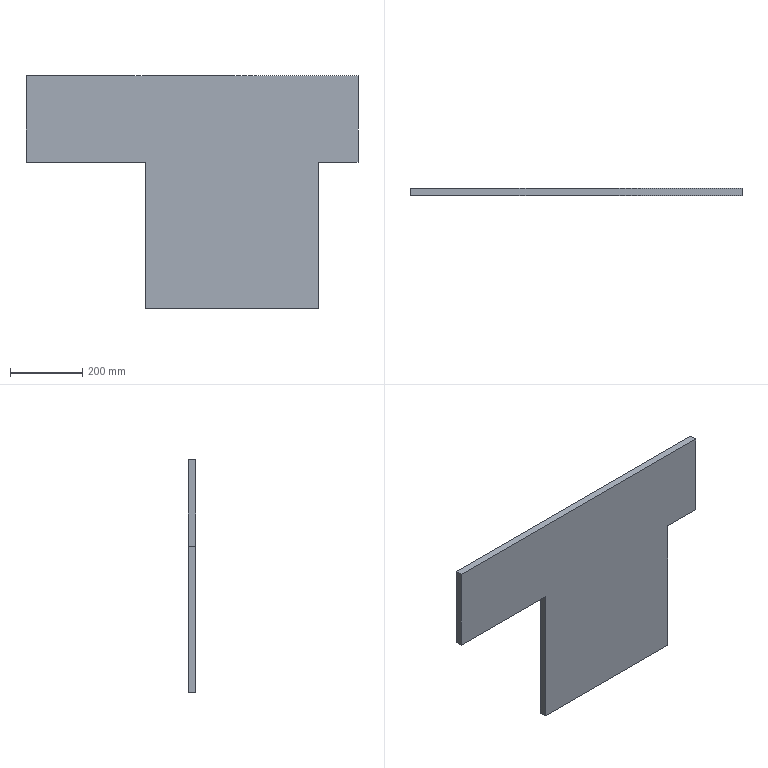Part | SolidWorks | features Extrusion 1 | 1 solid | 10 faces | box 920 x 20 x 645 mm | volume 8304000 mm3 | plane 10
STEP:
#1=CARTESIAN_POINT('',(590.,0.,655.));
#2=VERTEX_POINT('',#1);
#3=CARTESIAN_POINT('',(590.,0.,415.));
#4=VERTEX_POINT('',#3);
#5=CARTESIAN_POINT('',(590.,0.,655.));
#6=DIRECTION('',(0.,0.,-1.));
#7=VECTOR('',#6,1000.);
#8=LINE('',#5,#7);
#9=EDGE_CURVE('',#2,#4,#8,.T.);
#10=ORIENTED_EDGE('',*,*,#9,.T.);
#11=CARTESIAN_POINT('',(590.,20.,415.));
#12=VERTEX_POINT('',#11);
#13=CARTESIAN_POINT('',(590.,20.,415.));
#14=DIRECTION('',(0.,-1.,0.));
#15=VECTOR('',#14,1000.);
#16=LINE('',#13,#15);
#17=EDGE_CURVE('',#12,#4,#16,.T.);
#18=ORIENTED_EDGE('',*,*,#17,.F.);
#19=CARTESIAN_POINT('',(590.,20.,655.));
#20=VERTEX_POINT('',#19);
#21=CARTESIAN_POINT('',(590.,20.,655.));
#22=DIRECTION('',(0.,0.,-1.));
#23=VECTOR('',#22,1000.);
#24=LINE('',#21,#23);
#25=EDGE_CURVE('',#20,#12,#24,.T.);
#26=ORIENTED_EDGE('',*,*,#25,.F.);
#27=CARTESIAN_POINT('',(590.,20.,655.));
#28=DIRECTION('',(0.,-1.,0.));
#29=VECTOR('',#28,1000.);
#30=LINE('',#27,#29);
#31=EDGE_CURVE('',#20,#2,#30,.T.);
#32=ORIENTED_EDGE('',*,*,#31,.T.);
#33=EDGE_LOOP('',(#10,#18,#26,#32));
#34=FACE_OUTER_BOUND('',#33,.T.);
#35=CARTESIAN_POINT('',(590.,20.,655.));
#36=DIRECTION('',(-1.,0.,0.));
#37=DIRECTION('',(0.,0.,1.));
#38=AXIS2_PLACEMENT_3D('',#35,#36,#37);
#39=PLANE('',#38);
#40=ADVANCED_FACE('',(#34),#39,.F.);
#41=CARTESIAN_POINT('',(480.,0.,415.));
#42=VERTEX_POINT('',#41);
#43=CARTESIAN_POINT('',(590.,0.,415.));
#44=DIRECTION('',(-1.,0.,0.));
#45=VECTOR('',#44,1000.);
#46=LINE('',#43,#45);
#47=EDGE_CURVE('',#4,#42,#46,.T.);
#48=ORIENTED_EDGE('',*,*,#47,.T.);
#49=CARTESIAN_POINT('',(480.,20.,415.));
#50=VERTEX_POINT('',#49);
#51=CARTESIAN_POINT('',(480.,20.,415.));
#52=DIRECTION('',(0.,-1.,0.));
#53=VECTOR('',#52,1000.);
#54=LINE('',#51,#53);
#55=EDGE_CURVE('',#50,#42,#54,.T.);
#56=ORIENTED_EDGE('',*,*,#55,.F.);
#57=CARTESIAN_POINT('',(590.,20.,415.));
#58=DIRECTION('',(-1.,0.,0.));
#59=VECTOR('',#58,1000.);
#60=LINE('',#57,#59);
#61=EDGE_CURVE('',#12,#50,#60,.T.);
#62=ORIENTED_EDGE('',*,*,#61,.F.);
#63=ORIENTED_EDGE('',*,*,#17,.T.);
#64=EDGE_LOOP('',(#48,#56,#62,#63));
#65=FACE_OUTER_BOUND('',#64,.T.);
#66=CARTESIAN_POINT('',(590.,20.,415.));
#67=DIRECTION('',(0.,0.,1.));
#68=DIRECTION('',(1.,0.,0.));
#69=AXIS2_PLACEMENT_3D('',#66,#67,#68);
#70=PLANE('',#69);
#71=ADVANCED_FACE('',(#65),#70,.F.);
#72=CARTESIAN_POINT('',(480.,0.,10.));
#73=VERTEX_POINT('',#72);
#74=CARTESIAN_POINT('',(480.,0.,10.));
#75=DIRECTION('',(0.,0.,-1.));
#76=VECTOR('',#75,1000.);
#77=LINE('',#74,#76);
#78=EDGE_CURVE('',#42,#73,#77,.T.);
#79=ORIENTED_EDGE('',*,*,#78,.T.);
#80=CARTESIAN_POINT('',(480.,20.,10.));
#81=VERTEX_POINT('',#80);
#82=CARTESIAN_POINT('',(480.,20.,10.));
#83=DIRECTION('',(0.,-1.,0.));
#84=VECTOR('',#83,1000.);
#85=LINE('',#82,#84);
#86=EDGE_CURVE('',#81,#73,#85,.T.);
#87=ORIENTED_EDGE('',*,*,#86,.F.);
#88=CARTESIAN_POINT('',(480.,20.,10.));
#89=DIRECTION('',(0.,0.,-1.));
#90=VECTOR('',#89,1000.);
#91=LINE('',#88,#90);
#92=EDGE_CURVE('',#50,#81,#91,.T.);
#93=ORIENTED_EDGE('',*,*,#92,.F.);
#94=ORIENTED_EDGE('',*,*,#55,.T.);
#95=EDGE_LOOP('',(#79,#87,#93,#94));
#96=FACE_OUTER_BOUND('',#95,.T.);
#97=CARTESIAN_POINT('',(480.,20.,10.));
#98=DIRECTION('',(-1.,0.,0.));
#99=DIRECTION('',(0.,0.,1.));
#100=AXIS2_PLACEMENT_3D('',#97,#98,#99);
#101=PLANE('',#100);
#102=ADVANCED_FACE('',(#96),#101,.F.);
#103=CARTESIAN_POINT('',(0.,0.,10.));
#104=VERTEX_POINT('',#103);
#105=CARTESIAN_POINT('',(480.,0.,10.));
#106=DIRECTION('',(-1.,0.,0.));
#107=VECTOR('',#106,1000.);
#108=LINE('',#105,#107);
#109=EDGE_CURVE('',#73,#104,#108,.T.);
#110=ORIENTED_EDGE('',*,*,#109,.T.);
#111=CARTESIAN_POINT('',(0.,20.,10.));
#112=VERTEX_POINT('',#111);
#113=CARTESIAN_POINT('',(0.,20.,10.));
#114=DIRECTION('',(0.,-1.,0.));
#115=VECTOR('',#114,1000.);
#116=LINE('',#113,#115);
#117=EDGE_CURVE('',#112,#104,#116,.T.);
#118=ORIENTED_EDGE('',*,*,#117,.F.);
#119=CARTESIAN_POINT('',(480.,20.,10.));
#120=DIRECTION('',(-1.,0.,0.));
#121=VECTOR('',#120,1000.);
#122=LINE('',#119,#121);
#123=EDGE_CURVE('',#81,#112,#122,.T.);
#124=ORIENTED_EDGE('',*,*,#123,.F.);
#125=ORIENTED_EDGE('',*,*,#86,.T.);
#126=EDGE_LOOP('',(#110,#118,#124,#125));
#127=FACE_OUTER_BOUND('',#126,.T.);
#128=CARTESIAN_POINT('',(480.,20.,10.));
#129=DIRECTION('',(0.,0.,1.));
#130=DIRECTION('',(1.,0.,0.));
#131=AXIS2_PLACEMENT_3D('',#128,#129,#130);
#132=PLANE('',#131);
#133=ADVANCED_FACE('',(#127),#132,.F.);
#134=CARTESIAN_POINT('',(0.,0.,415.));
#135=VERTEX_POINT('',#134);
#136=CARTESIAN_POINT('',(0.,0.,415.));
#137=DIRECTION('',(0.,0.,1.));
#138=VECTOR('',#137,1000.);
#139=LINE('',#136,#138);
#140=EDGE_CURVE('',#104,#135,#139,.T.);
#141=ORIENTED_EDGE('',*,*,#140,.T.);
#142=CARTESIAN_POINT('',(0.,20.,415.));
#143=VERTEX_POINT('',#142);
#144=CARTESIAN_POINT('',(0.,20.,415.));
#145=DIRECTION('',(0.,-1.,0.));
#146=VECTOR('',#145,1000.);
#147=LINE('',#144,#146);
#148=EDGE_CURVE('',#143,#135,#147,.T.);
#149=ORIENTED_EDGE('',*,*,#148,.F.);
#150=CARTESIAN_POINT('',(0.,20.,415.));
#151=DIRECTION('',(0.,0.,1.));
#152=VECTOR('',#151,1000.);
#153=LINE('',#150,#152);
#154=EDGE_CURVE('',#112,#143,#153,.T.);
#155=ORIENTED_EDGE('',*,*,#154,.F.);
#156=ORIENTED_EDGE('',*,*,#117,.T.);
#157=EDGE_LOOP('',(#141,#149,#155,#156));
#158=FACE_OUTER_BOUND('',#157,.T.);
#159=CARTESIAN_POINT('',(0.,20.,415.));
#160=DIRECTION('',(1.,0.,0.));
#161=DIRECTION('',(0.,0.,-1.));
#162=AXIS2_PLACEMENT_3D('',#159,#160,#161);
#163=PLANE('',#162);
#164=ADVANCED_FACE('',(#158),#163,.F.);
#165=CARTESIAN_POINT('',(-330.,0.,415.));
#166=VERTEX_POINT('',#165);
#167=CARTESIAN_POINT('',(0.,0.,415.));
#168=DIRECTION('',(-1.,0.,0.));
#169=VECTOR('',#168,1000.);
#170=LINE('',#167,#169);
#171=EDGE_CURVE('',#135,#166,#170,.T.);
#172=ORIENTED_EDGE('',*,*,#171,.T.);
#173=CARTESIAN_POINT('',(-330.,20.,415.));
#174=VERTEX_POINT('',#173);
#175=CARTESIAN_POINT('',(-330.,20.,415.));
#176=DIRECTION('',(0.,-1.,0.));
#177=VECTOR('',#176,1000.);
#178=LINE('',#175,#177);
#179=EDGE_CURVE('',#174,#166,#178,.T.);
#180=ORIENTED_EDGE('',*,*,#179,.F.);
#181=CARTESIAN_POINT('',(0.,20.,415.));
#182=DIRECTION('',(-1.,0.,0.));
#183=VECTOR('',#182,1000.);
#184=LINE('',#181,#183);
#185=EDGE_CURVE('',#143,#174,#184,.T.);
#186=ORIENTED_EDGE('',*,*,#185,.F.);
#187=ORIENTED_EDGE('',*,*,#148,.T.);
#188=EDGE_LOOP('',(#172,#180,#186,#187));
#189=FACE_OUTER_BOUND('',#188,.T.);
#190=CARTESIAN_POINT('',(0.,20.,415.));
#191=DIRECTION('',(0.,0.,1.));
#192=DIRECTION('',(1.,0.,0.));
#193=AXIS2_PLACEMENT_3D('',#190,#191,#192);
#194=PLANE('',#193);
#195=ADVANCED_FACE('',(#189),#194,.F.);
#196=CARTESIAN_POINT('',(-330.,0.,655.));
#197=VERTEX_POINT('',#196);
#198=CARTESIAN_POINT('',(-330.,0.,415.));
#199=DIRECTION('',(0.,0.,1.));
#200=VECTOR('',#199,1000.);
#201=LINE('',#198,#200);
#202=EDGE_CURVE('',#166,#197,#201,.T.);
#203=ORIENTED_EDGE('',*,*,#202,.T.);
#204=CARTESIAN_POINT('',(-330.,20.,655.));
#205=VERTEX_POINT('',#204);
#206=CARTESIAN_POINT('',(-330.,20.,655.));
#207=DIRECTION('',(0.,-1.,0.));
#208=VECTOR('',#207,1000.);
#209=LINE('',#206,#208);
#210=EDGE_CURVE('',#205,#197,#209,.T.);
#211=ORIENTED_EDGE('',*,*,#210,.F.);
#212=CARTESIAN_POINT('',(-330.,20.,415.));
#213=DIRECTION('',(0.,0.,1.));
#214=VECTOR('',#213,1000.);
#215=LINE('',#212,#214);
#216=EDGE_CURVE('',#174,#205,#215,.T.);
#217=ORIENTED_EDGE('',*,*,#216,.F.);
#218=ORIENTED_EDGE('',*,*,#179,.T.);
#219=EDGE_LOOP('',(#203,#211,#217,#218));
#220=FACE_OUTER_BOUND('',#219,.T.);
#221=CARTESIAN_POINT('',(-330.,20.,415.));
#222=DIRECTION('',(1.,0.,0.));
#223=DIRECTION('',(0.,0.,-1.));
#224=AXIS2_PLACEMENT_3D('',#221,#222,#223);
#225=PLANE('',#224);
#226=ADVANCED_FACE('',(#220),#225,.F.);
#227=CARTESIAN_POINT('',(-330.,0.,655.));
#228=DIRECTION('',(1.,0.,0.));
#229=VECTOR('',#228,1000.);
#230=LINE('',#227,#229);
#231=EDGE_CURVE('',#197,#2,#230,.T.);
#232=ORIENTED_EDGE('',*,*,#231,.T.);
#233=ORIENTED_EDGE('',*,*,#31,.F.);
#234=CARTESIAN_POINT('',(-330.,20.,655.));
#235=DIRECTION('',(1.,0.,0.));
#236=VECTOR('',#235,1000.);
#237=LINE('',#234,#236);
#238=EDGE_CURVE('',#205,#20,#237,.T.);
#239=ORIENTED_EDGE('',*,*,#238,.F.);
#240=ORIENTED_EDGE('',*,*,#210,.T.);
#241=EDGE_LOOP('',(#232,#233,#239,#240));
#242=FACE_OUTER_BOUND('',#241,.T.);
#243=CARTESIAN_POINT('',(-330.,20.,655.));
#244=DIRECTION('',(0.,0.,-1.));
#245=DIRECTION('',(-1.,0.,0.));
#246=AXIS2_PLACEMENT_3D('',#243,#244,#245);
#247=PLANE('',#246);
#248=ADVANCED_FACE('',(#242),#247,.F.);
#249=ORIENTED_EDGE('',*,*,#25,.T.);
#250=ORIENTED_EDGE('',*,*,#61,.T.);
#251=ORIENTED_EDGE('',*,*,#92,.T.);
#252=ORIENTED_EDGE('',*,*,#123,.T.);
#253=ORIENTED_EDGE('',*,*,#154,.T.);
#254=ORIENTED_EDGE('',*,*,#185,.T.);
#255=ORIENTED_EDGE('',*,*,#216,.T.);
#256=ORIENTED_EDGE('',*,*,#238,.T.);
#257=EDGE_LOOP('',(#249,#250,#251,#252,#253,#254,#255,#256));
#258=FACE_OUTER_BOUND('',#257,.T.);
#259=CARTESIAN_POINT('',(0.,20.,0.));
#260=DIRECTION('',(0.,1.,0.));
#261=DIRECTION('',(0.,0.,1.));
#262=AXIS2_PLACEMENT_3D('',#259,#260,#261);
#263=PLANE('',#262);
#264=ADVANCED_FACE('',(#258),#263,.T.);
#265=ORIENTED_EDGE('',*,*,#9,.F.);
#266=ORIENTED_EDGE('',*,*,#231,.F.);
#267=ORIENTED_EDGE('',*,*,#202,.F.);
#268=ORIENTED_EDGE('',*,*,#171,.F.);
#269=ORIENTED_EDGE('',*,*,#140,.F.);
#270=ORIENTED_EDGE('',*,*,#109,.F.);
#271=ORIENTED_EDGE('',*,*,#78,.F.);
#272=ORIENTED_EDGE('',*,*,#47,.F.);
#273=EDGE_LOOP('',(#265,#266,#267,#268,#269,#270,#271,#272));
#274=FACE_OUTER_BOUND('',#273,.T.);
#275=CARTESIAN_POINT('',(0.,0.,0.));
#276=DIRECTION('',(0.,1.,0.));
#277=DIRECTION('',(0.,0.,1.));
#278=AXIS2_PLACEMENT_3D('',#275,#276,#277);
#279=PLANE('',#278);
#280=ADVANCED_FACE('',(#274),#279,.F.);
#281=CLOSED_SHELL('',(#40,#71,#102,#133,#164,#195,#226,#248,#264,#280));
#282=MANIFOLD_SOLID_BREP('',#281);
#283=CARTESIAN_POINT('',(0.,0.,0.));
#284=DIRECTION('',(0.,0.,1.));
#285=DIRECTION('',(1.,0.,0.));
#286=AXIS2_PLACEMENT_3D('',#283,#284,#285);
#287=(LENGTH_UNIT()NAMED_UNIT(*)SI_UNIT(.MILLI.,.METRE.));
#288=UNCERTAINTY_MEASURE_WITH_UNIT(LENGTH_MEASURE(0.00001),#287,'','');
#289=(NAMED_UNIT(*)PLANE_ANGLE_UNIT()SI_UNIT($,.RADIAN.));
#290=(NAMED_UNIT(*)SI_UNIT($,.STERADIAN.)SOLID_ANGLE_UNIT());
#291=(GEOMETRIC_REPRESENTATION_CONTEXT(3)GLOBAL_UNCERTAINTY_ASSIGNED_CONTEXT((#288))GLOBAL_UNIT_ASSIGNED_CONTEXT((#287,#289,#290))REPRESENTATION_CONTEXT('',''));
#292=ADVANCED_BREP_SHAPE_REPRESENTATION('',(#282,#286),#291);